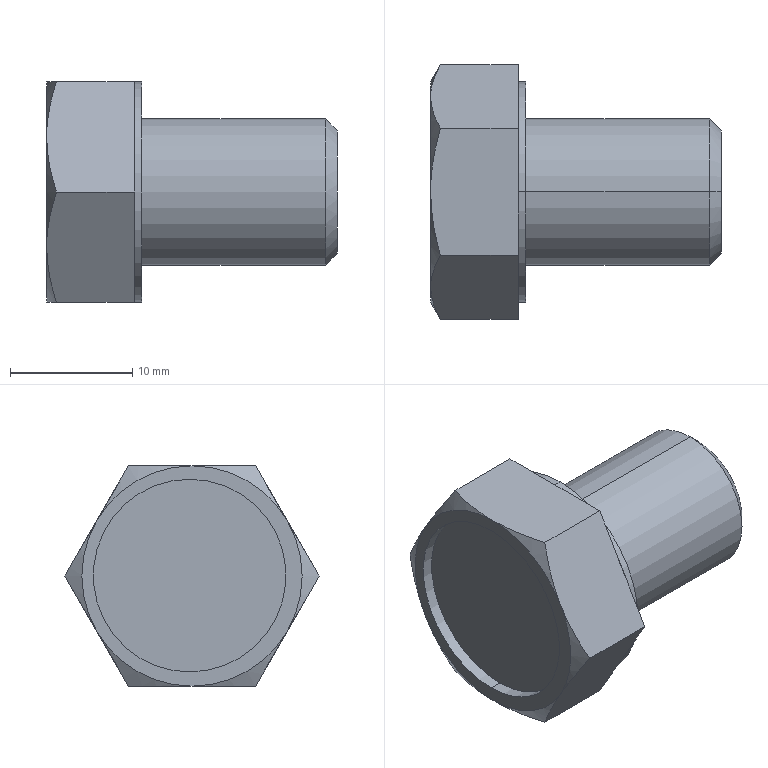Part | STEP file | formed hex screw_am_B18.2.3.2M - Formed hex screw, M12 x 1.75 x 16 --16WN | 1 solid | 30 faces | box 23.76 x 20.785 x 18 mm | volume 3759 mm3 | plane 16 | cone 8 | cylinder 6 | commonest cylinder face diameters 12 x2 15.75 x2 18 x2